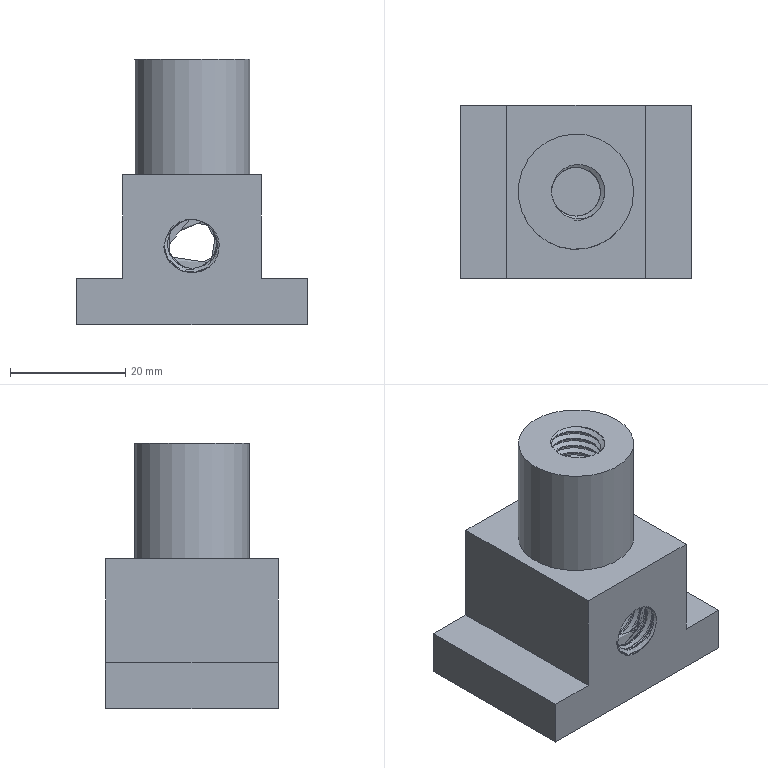Part | NX | features DATUM_CSYS 3, HOLE PACKAGE 2, SIMPLE HOLE 2, SKETCH 2, THREADS 2, BLOCK 1, CYLINDER 1, EXTRUDE 1, UNITE 1 | 1 solid | 33 faces | box 40 x 30 x 46 mm | volume 25067 mm3 | cylinder 15 | plane 14 | spline 4 | commonest cylinder face diameters 8.5 x12 10 x2 20 x1